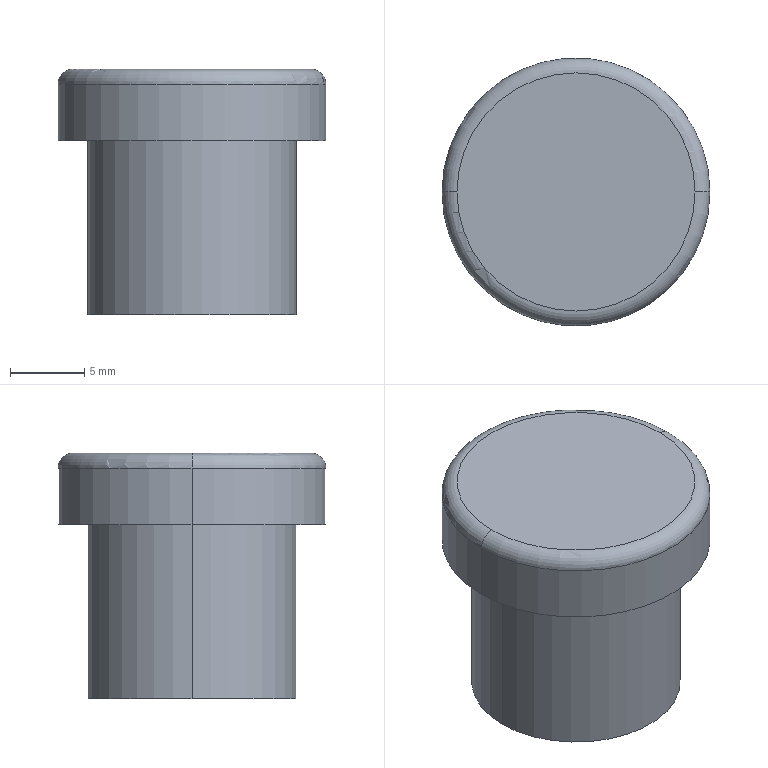Part | SolidWorks | features BaseBody 1 | 1 solid | 9 faces | box 18 x 18 x 16.5 mm | volume 3011 mm3 | cylinder 4 | plane 3 | torus 2 | commonest cylinder face diameters 14 x2 18 x2
STEP:
#1=CARTESIAN_POINT('',(8.,0.,16.5));
#2=VERTEX_POINT('',#1);
#3=CARTESIAN_POINT('',(-8.,0.,16.5));
#4=VERTEX_POINT('',#3);
#5=CARTESIAN_POINT('',(0.,0.,16.5));
#6=DIRECTION('',(0.,0.,-1.));
#7=DIRECTION('',(1.,0.,0.));
#8=AXIS2_PLACEMENT_3D('',#5,#6,#7);
#9=CIRCLE('',#8,8.);
#10=EDGE_CURVE('',#2,#4,#9,.T.);
#11=ORIENTED_EDGE('',*,*,#10,.F.);
#12=CARTESIAN_POINT('',(0.,0.,16.5));
#13=DIRECTION('',(0.,0.,-1.));
#14=DIRECTION('',(-1.,0.,0.));
#15=AXIS2_PLACEMENT_3D('',#12,#13,#14);
#16=CIRCLE('',#15,8.);
#17=EDGE_CURVE('',#4,#2,#16,.T.);
#18=ORIENTED_EDGE('',*,*,#17,.F.);
#19=EDGE_LOOP('',(#11,#18));
#20=FACE_OUTER_BOUND('',#19,.T.);
#21=CARTESIAN_POINT('',(0.,0.,16.5));
#22=DIRECTION('',(0.,0.,1.));
#23=DIRECTION('',(1.,0.,0.));
#24=AXIS2_PLACEMENT_3D('',#21,#22,#23);
#25=PLANE('',#24);
#26=ADVANCED_FACE('',(#20),#25,.T.);
#27=CARTESIAN_POINT('',(-9.,0.,15.5));
#28=VERTEX_POINT('',#27);
#29=CARTESIAN_POINT('',(-8.,0.,15.5));
#30=DIRECTION('',(0.,1.,0.));
#31=DIRECTION('',(-1.,0.,0.));
#32=AXIS2_PLACEMENT_3D('',#29,#30,#31);
#33=CIRCLE('',#32,1.);
#34=EDGE_CURVE('',#28,#4,#33,.T.);
#35=ORIENTED_EDGE('',*,*,#34,.T.);
#36=ORIENTED_EDGE('',*,*,#17,.T.);
#37=CARTESIAN_POINT('',(9.,0.,15.5));
#38=VERTEX_POINT('',#37);
#39=CARTESIAN_POINT('',(8.,0.,15.5));
#40=DIRECTION('',(0.,-1.,0.));
#41=DIRECTION('',(1.,0.,0.));
#42=AXIS2_PLACEMENT_3D('',#39,#40,#41);
#43=CIRCLE('',#42,1.);
#44=EDGE_CURVE('',#38,#2,#43,.T.);
#45=ORIENTED_EDGE('',*,*,#44,.F.);
#46=CARTESIAN_POINT('',(0.,0.,15.5));
#47=DIRECTION('',(0.,0.,-1.));
#48=DIRECTION('',(-1.,0.,0.));
#49=AXIS2_PLACEMENT_3D('',#46,#47,#48);
#50=CIRCLE('',#49,9.);
#51=EDGE_CURVE('',#28,#38,#50,.T.);
#52=ORIENTED_EDGE('',*,*,#51,.F.);
#53=EDGE_LOOP('',(#35,#36,#45,#52));
#54=FACE_OUTER_BOUND('',#53,.T.);
#55=CARTESIAN_POINT('',(0.,0.,15.5));
#56=DIRECTION('',(0.,0.,1.));
#57=DIRECTION('',(1.,0.,0.));
#58=AXIS2_PLACEMENT_3D('',#55,#56,#57);
#59=TOROIDAL_SURFACE('',#58,8.,1.);
#60=ADVANCED_FACE('',(#54),#59,.T.);
#61=CARTESIAN_POINT('',(9.,0.,11.7));
#62=VERTEX_POINT('',#61);
#63=CARTESIAN_POINT('',(9.,0.,15.5));
#64=DIRECTION('',(0.,0.,-1.));
#65=VECTOR('',#64,1000.);
#66=LINE('',#63,#65);
#67=EDGE_CURVE('',#38,#62,#66,.T.);
#68=ORIENTED_EDGE('',*,*,#67,.T.);
#69=CARTESIAN_POINT('',(-9.,0.,11.7));
#70=VERTEX_POINT('',#69);
#71=CARTESIAN_POINT('',(0.,0.,11.7));
#72=DIRECTION('',(0.,0.,1.));
#73=DIRECTION('',(1.,0.,0.));
#74=AXIS2_PLACEMENT_3D('',#71,#72,#73);
#75=CIRCLE('',#74,9.);
#76=EDGE_CURVE('',#62,#70,#75,.T.);
#77=ORIENTED_EDGE('',*,*,#76,.T.);
#78=CARTESIAN_POINT('',(-9.,0.,15.5));
#79=DIRECTION('',(0.,0.,-1.));
#80=VECTOR('',#79,1000.);
#81=LINE('',#78,#80);
#82=EDGE_CURVE('',#28,#70,#81,.T.);
#83=ORIENTED_EDGE('',*,*,#82,.F.);
#84=ORIENTED_EDGE('',*,*,#51,.T.);
#85=EDGE_LOOP('',(#68,#77,#83,#84));
#86=FACE_OUTER_BOUND('',#85,.T.);
#87=CARTESIAN_POINT('',(0.,0.,16.5));
#88=DIRECTION('',(0.,0.,-1.));
#89=DIRECTION('',(-1.,0.,0.));
#90=AXIS2_PLACEMENT_3D('',#87,#88,#89);
#91=CYLINDRICAL_SURFACE('',#90,9.);
#92=ADVANCED_FACE('',(#86),#91,.T.);
#93=CARTESIAN_POINT('',(0.,0.,15.5));
#94=DIRECTION('',(0.,0.,-1.));
#95=DIRECTION('',(1.,0.,0.));
#96=AXIS2_PLACEMENT_3D('',#93,#94,#95);
#97=CIRCLE('',#96,9.);
#98=EDGE_CURVE('',#38,#28,#97,.T.);
#99=ORIENTED_EDGE('',*,*,#98,.T.);
#100=ORIENTED_EDGE('',*,*,#82,.T.);
#101=CARTESIAN_POINT('',(0.,0.,11.7));
#102=DIRECTION('',(0.,0.,1.));
#103=DIRECTION('',(-1.,0.,0.));
#104=AXIS2_PLACEMENT_3D('',#101,#102,#103);
#105=CIRCLE('',#104,9.);
#106=EDGE_CURVE('',#70,#62,#105,.T.);
#107=ORIENTED_EDGE('',*,*,#106,.T.);
#108=ORIENTED_EDGE('',*,*,#67,.F.);
#109=EDGE_LOOP('',(#99,#100,#107,#108));
#110=FACE_OUTER_BOUND('',#109,.T.);
#111=CARTESIAN_POINT('',(0.,0.,16.5));
#112=DIRECTION('',(0.,0.,-1.));
#113=DIRECTION('',(-1.,0.,0.));
#114=AXIS2_PLACEMENT_3D('',#111,#112,#113);
#115=CYLINDRICAL_SURFACE('',#114,9.);
#116=ADVANCED_FACE('',(#110),#115,.T.);
#117=CARTESIAN_POINT('',(-7.,0.,11.7));
#118=VERTEX_POINT('',#117);
#119=CARTESIAN_POINT('',(7.,0.,11.7));
#120=VERTEX_POINT('',#119);
#121=CARTESIAN_POINT('',(0.,0.,11.7));
#122=DIRECTION('',(0.,0.,-1.));
#123=DIRECTION('',(-1.,0.,0.));
#124=AXIS2_PLACEMENT_3D('',#121,#122,#123);
#125=CIRCLE('',#124,7.);
#126=EDGE_CURVE('',#118,#120,#125,.T.);
#127=ORIENTED_EDGE('',*,*,#126,.F.);
#128=CARTESIAN_POINT('',(0.,0.,11.7));
#129=DIRECTION('',(0.,0.,-1.));
#130=DIRECTION('',(1.,0.,0.));
#131=AXIS2_PLACEMENT_3D('',#128,#129,#130);
#132=CIRCLE('',#131,7.);
#133=EDGE_CURVE('',#120,#118,#132,.T.);
#134=ORIENTED_EDGE('',*,*,#133,.F.);
#135=EDGE_LOOP('',(#127,#134));
#136=FACE_BOUND('',#135,.T.);
#137=ORIENTED_EDGE('',*,*,#76,.F.);
#138=ORIENTED_EDGE('',*,*,#106,.F.);
#139=EDGE_LOOP('',(#137,#138));
#140=FACE_OUTER_BOUND('',#139,.T.);
#141=CARTESIAN_POINT('',(0.,0.,11.7));
#142=DIRECTION('',(0.,0.,1.));
#143=DIRECTION('',(1.,0.,0.));
#144=AXIS2_PLACEMENT_3D('',#141,#142,#143);
#145=PLANE('',#144);
#146=ADVANCED_FACE('',(#136,#140),#145,.F.);
#147=ORIENTED_EDGE('',*,*,#133,.T.);
#148=CARTESIAN_POINT('',(-7.,0.,0.));
#149=VERTEX_POINT('',#148);
#150=CARTESIAN_POINT('',(-7.,0.,11.7));
#151=DIRECTION('',(0.,0.,-1.));
#152=VECTOR('',#151,1000.);
#153=LINE('',#150,#152);
#154=EDGE_CURVE('',#118,#149,#153,.T.);
#155=ORIENTED_EDGE('',*,*,#154,.T.);
#156=CARTESIAN_POINT('',(7.,0.,0.));
#157=VERTEX_POINT('',#156);
#158=CARTESIAN_POINT('',(0.,0.,0.));
#159=DIRECTION('',(0.,0.,1.));
#160=DIRECTION('',(-1.,0.,0.));
#161=AXIS2_PLACEMENT_3D('',#158,#159,#160);
#162=CIRCLE('',#161,7.);
#163=EDGE_CURVE('',#149,#157,#162,.T.);
#164=ORIENTED_EDGE('',*,*,#163,.T.);
#165=CARTESIAN_POINT('',(7.,0.,11.7));
#166=DIRECTION('',(0.,0.,-1.));
#167=VECTOR('',#166,1000.);
#168=LINE('',#165,#167);
#169=EDGE_CURVE('',#120,#157,#168,.T.);
#170=ORIENTED_EDGE('',*,*,#169,.F.);
#171=EDGE_LOOP('',(#147,#155,#164,#170));
#172=FACE_OUTER_BOUND('',#171,.T.);
#173=CARTESIAN_POINT('',(0.,0.,11.7));
#174=DIRECTION('',(0.,0.,-1.));
#175=DIRECTION('',(-1.,0.,0.));
#176=AXIS2_PLACEMENT_3D('',#173,#174,#175);
#177=CYLINDRICAL_SURFACE('',#176,7.);
#178=ADVANCED_FACE('',(#172),#177,.T.);
#179=ORIENTED_EDGE('',*,*,#169,.T.);
#180=CARTESIAN_POINT('',(0.,0.,0.));
#181=DIRECTION('',(0.,0.,1.));
#182=DIRECTION('',(1.,0.,0.));
#183=AXIS2_PLACEMENT_3D('',#180,#181,#182);
#184=CIRCLE('',#183,7.);
#185=EDGE_CURVE('',#157,#149,#184,.T.);
#186=ORIENTED_EDGE('',*,*,#185,.T.);
#187=ORIENTED_EDGE('',*,*,#154,.F.);
#188=ORIENTED_EDGE('',*,*,#126,.T.);
#189=EDGE_LOOP('',(#179,#186,#187,#188));
#190=FACE_OUTER_BOUND('',#189,.T.);
#191=CARTESIAN_POINT('',(0.,0.,11.7));
#192=DIRECTION('',(0.,0.,-1.));
#193=DIRECTION('',(-1.,0.,0.));
#194=AXIS2_PLACEMENT_3D('',#191,#192,#193);
#195=CYLINDRICAL_SURFACE('',#194,7.);
#196=ADVANCED_FACE('',(#190),#195,.T.);
#197=ORIENTED_EDGE('',*,*,#185,.F.);
#198=ORIENTED_EDGE('',*,*,#163,.F.);
#199=EDGE_LOOP('',(#197,#198));
#200=FACE_OUTER_BOUND('',#199,.T.);
#201=CARTESIAN_POINT('',(0.,0.,0.));
#202=DIRECTION('',(0.,0.,1.));
#203=DIRECTION('',(1.,0.,0.));
#204=AXIS2_PLACEMENT_3D('',#201,#202,#203);
#205=PLANE('',#204);
#206=ADVANCED_FACE('',(#200),#205,.F.);
#207=ORIENTED_EDGE('',*,*,#98,.F.);
#208=ORIENTED_EDGE('',*,*,#44,.T.);
#209=ORIENTED_EDGE('',*,*,#10,.T.);
#210=ORIENTED_EDGE('',*,*,#34,.F.);
#211=EDGE_LOOP('',(#207,#208,#209,#210));
#212=FACE_OUTER_BOUND('',#211,.T.);
#213=CARTESIAN_POINT('',(0.,0.,15.5));
#214=DIRECTION('',(0.,0.,1.));
#215=DIRECTION('',(1.,0.,0.));
#216=AXIS2_PLACEMENT_3D('',#213,#214,#215);
#217=TOROIDAL_SURFACE('',#216,8.,1.);
#218=ADVANCED_FACE('',(#212),#217,.T.);
#219=CLOSED_SHELL('',(#26,#60,#92,#116,#146,#178,#196,#206,#218));
#220=MANIFOLD_SOLID_BREP('',#219);
#221=CARTESIAN_POINT('',(0.,0.,0.));
#222=DIRECTION('',(0.,0.,1.));
#223=DIRECTION('',(1.,0.,0.));
#224=AXIS2_PLACEMENT_3D('',#221,#222,#223);
#225=(LENGTH_UNIT()NAMED_UNIT(*)SI_UNIT(.MILLI.,.METRE.));
#226=UNCERTAINTY_MEASURE_WITH_UNIT(LENGTH_MEASURE(0.00001),#225,'','');
#227=(NAMED_UNIT(*)PLANE_ANGLE_UNIT()SI_UNIT($,.RADIAN.));
#228=(NAMED_UNIT(*)SI_UNIT($,.STERADIAN.)SOLID_ANGLE_UNIT());
#229=(GEOMETRIC_REPRESENTATION_CONTEXT(3)GLOBAL_UNCERTAINTY_ASSIGNED_CONTEXT((#226))GLOBAL_UNIT_ASSIGNED_CONTEXT((#225,#227,#228))REPRESENTATION_CONTEXT('',''));
#230=ADVANCED_BREP_SHAPE_REPRESENTATION('',(#220,#224),#229);